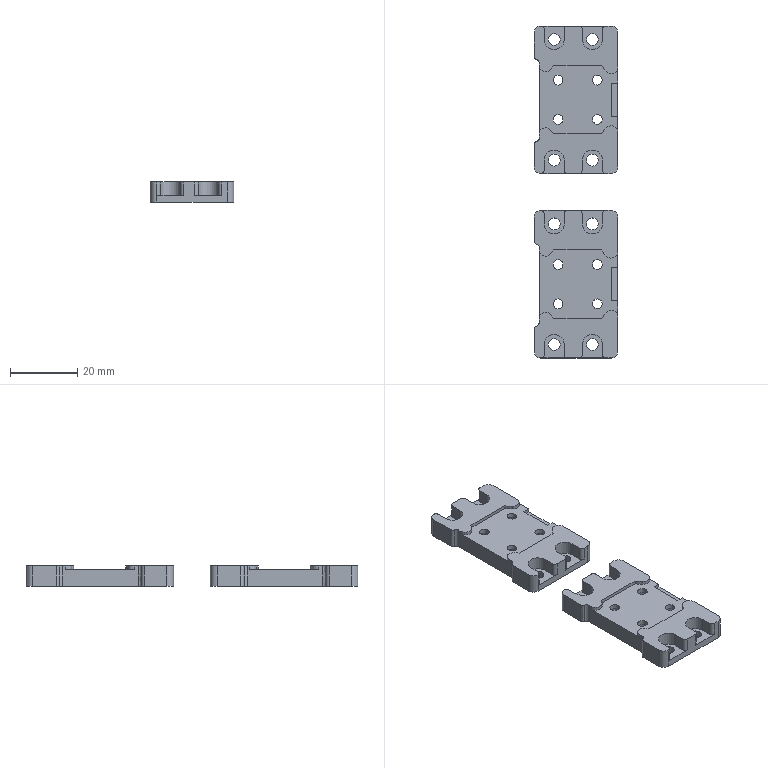CAM job | NX | 3-axis milling, drilling | part box 25 x 99 x 6 mm | stock box 30 x 104 x 8 mm
Tools:
number,name,description,diameter,corner_radius,flute_length,length,flutes
3,D3,平底铣刀-粗,3.0,0.0,20.0,75.0,2
4,D4,平底铣刀-粗,4.0,0.0,25.0,75.0,2
9,D10,平底铣刀-粗,10.0,0.0,35.0,75.0,2
19,D2-J,平底铣刀-精,2.0,0.0,50.0,75.0,2
17,D3-J,平底铣刀-精,3.0,0.0,50.0,75.0,2
11,D4-J,平底铣刀-精,4.0,0.0,50.0,75.0,2
7,D6-J,平底铣刀-精,6.0,0.0,25.0,75.0,2
1,D80R0.8飞刀,圆鼻刀-粗,80.0,0.8,50.0,75.0,2
1,D80R0.8飞刀-J,圆鼻刀-精,80.0,0.8,50.0,75.0,2
2,D6倒角刀,倒角刀,6.0,0.0,3.0,25.0,2
18,ZT3.5,钻头,3.5,0.0,35.0,50.0,2
17,ZT2.9,Drilling Tool,2.9,0.0,35.0,50.0,2
Operations:
program,operation,operation_type,tool,method,geometry_group,spindle_rpm,surface_speed,feed_per_tooth,feed_cut,feed_plunge,cut_length_mm,path_length_mm,cut_time_min,machine_time_min
B,底壁铣飞面一刀开粗_COPY,VolumeBased25DMillingOperation,D80R0.8飞刀,分层开粗-切深K-步距G,W-B,2800.0,703.696,0.5357,3000.0,100.0,828.921,1472.989,0.2763,0.3407
B,底壁铣飞面一刀精光_COPY,VolumeBased25DMillingOperation,D80R0.8飞刀-J,侧刃精光-切深K-步距G,W-B,4000.0,1005.28,0.125,1000.0,100.0,207.034,243.034,0.207,0.2106
B,铣沉头_1,CylinderMilling,D3,METHOD,W-B,8000.0,75.398,0.0688,1100.0,100.0,1069.783,1418.803,0.9725,1.007
B,铣沉头_2,CylinderMilling,D3,METHOD,W-B,8000.0,75.398,0.0688,1100.0,100.0,368.642,508.042,0.3351,0.3491
B,钻倒角_3,Operation,D6倒角刀,METHOD,W-B,8000.0,150.796,0.0625,1000.0,0.0,40.4,280.362,0.0404,0.0644
B,C0.3封闭铣廓倒角6X45L_COPY,PlanarMilling,D6倒角刀,爬面_倒角-切深0-步距G,W-B,7000.0,131.0,0.0357,500.0,100.0,230.659,635.216,0.4613,0.5018
B,C0.3封闭铣廓倒角6X45L_COPY_1,PlanarMilling,D6倒角刀,爬面_倒角-切深0-步距G,W-B,7000.0,131.0,0.1071,1500.0,100.0,307.195,424.26,0.2048,0.2165
B,铣孔_1,CylinderMilling,D3-J,METHOD,W-B,8000.0,75.398,0.0187,300.0,100.0,124.988,501.808,0.4166,0.4543
B,铣孔_2,CylinderMilling,D3-J,METHOD,W-B,8000.0,75.398,0.0187,300.0,100.0,45.45,194.45,0.1515,0.1664
A,顶面,FaceMilling,D80R0.8飞刀,侧刃精光-切深K-步距G,W-A,4000.0,1005.31,0.125,1000.0,100.0,193.0,229.0,0.193,0.1966
A,外形粗_2,VolumeBased25DMillingOperation,D10,METHOD,W-A,8000.0,251.327,0.3125,5000.0,80.0,3349.822,3494.522,0.67,0.6844
A,打点-深0.8,Operation,D6倒角刀,NONE,W-A,8000.0,150.796,0.0312,500.0,90.0,28.8,296.742,0.0576,0.0844
A,通孔-2-3,Operation,ZT2.9,NONE,W-A,3000.0,27.332,0.0133,80.0,90.0,64.0,288.588,0.8,0.8225
A,通孔-3-4,Operation,ZT3.5,NONE,W-A,3000.0,32.987,0.02,120.0,90.0,80.412,344.576,0.6701,0.6965
A,底壁粗_1,VolumeBased25DMillingOperation,D4,METHOD,W-A,8000.0,100.531,0.2188,3500.0,100.0,1533.589,1746.734,0.4382,0.4595
A,底壁粗_2,VolumeBased25DMillingOperation,D4,METHOD,W-A,8000.0,100.531,0.075,1200.0,100.0,2598.509,3742.048,2.165,2.28
A,底壁粗_3,VolumeBased25DMillingOperation,D3,METHOD,W-A,6000.0,56.549,0.0833,1000.0,100.0,207.0,383.979,0.207,0.2247
A,底精_1,VolumeBased25DMillingOperation,D4-J,METHOD,W-A,6000.0,113.0,0.2083,1200.0,100.0,379.617,519.973,0.3163,0.3304
A,底侧精_3,VolumeBased25DMillingOperation,D4-J,METHOD,W-A,6000.0,113.0,0.2083,1200.0,100.0,163.498,439.322,0.1362,0.1638
A,底侧精_4,VolumeBased25DMillingOperation,D4-J,METHOD,W-A,6000.0,113.0,0.2083,1200.0,100.0,200.5,591.947,0.1671,0.2062
A,等高光顺清角D2参考6_COPY_COPY,ZLevelMilling,D2-J,分层精光-切深K-步距G,W-A,8000.0,50.264,0.05,800.0,100.0,178.375,333.562,0.223,0.2385
A,外形侧面,ZLevelMilling,D2-J,METHOD,W-A,9000.0,56.549,0.0833,1500.0,80.0,791.852,984.43,0.5289,0.5482
A,等高光顺清角D2参考6_COPY,ZLevelMilling,D2-J,分层精光-切深K-步距G,W-A,8000.0,50.264,0.05,800.0,100.0,471.199,731.321,0.589,0.615
A,底精_3,VolumeBased25DMillingOperation,D2-J,METHOD,W-A,6000.0,113.0,0.0667,800.0,100.0,51.4,192.9,0.0642,0.0784
A,底侧精_5,VolumeBased25DMillingOperation,D2-J,METHOD,W-A,6000.0,113.0,0.0667,800.0,100.0,32.283,179.063,0.0404,0.055
A,仅选体,SurfaceContour,D6倒角刀,METHOD,W-A,8000.0,150.796,0.1875,3000.0,100.0,567.674,1194.288,0.1892,0.2519
A,钻倒角_1,Operation,D6倒角刀,METHOD,W-A,8000.0,150.796,0.0312,500.0,0.0,38.0,254.701,0.076,0.0977
A,钻倒角_2,Operation,D6倒角刀,METHOD,W-A,8000.0,150.796,0.0312,500.0,0.0,40.4,288.362,0.0808,0.1056
A,外形半精_2,VolumeBased25DMillingOperation,D6-J,METHOD,W-A,8000.0,251.327,0.0625,1000.0,100.0,318.589,478.502,0.3186,0.3346